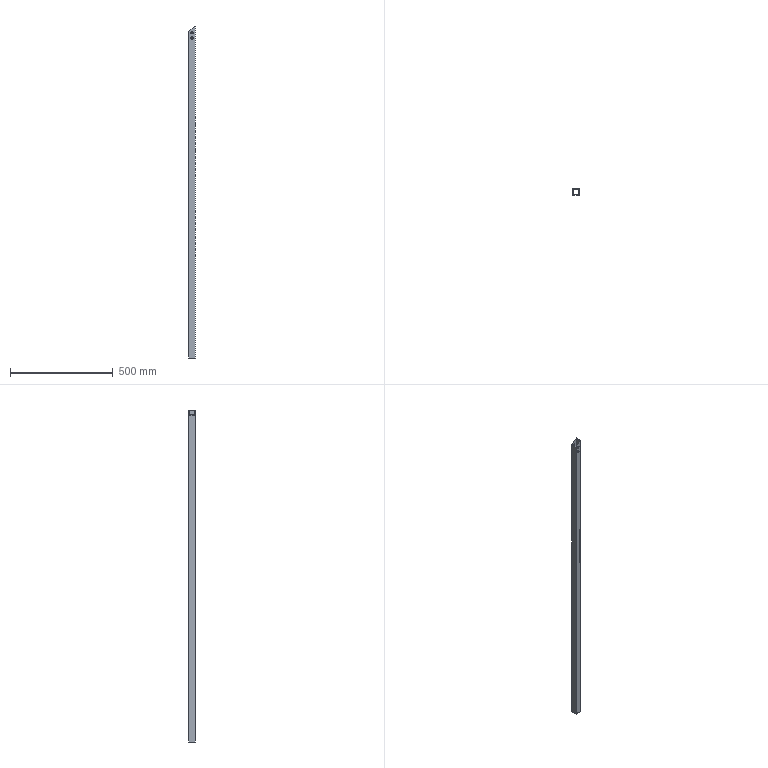Part | SolidWorks | features Cut 1, Extrusion 1, ICE 1 | 1 solid | 18 faces | box 30 x 30 x 1612 mm | volume 357438 mm3 | plane 10 | cylinder 8 | commonest cylinder face diameters 11.5 x8
STEP:
#1=CARTESIAN_POINT('',(-5.75,15.,745.414));
#2=VERTEX_POINT('',#1);
#3=CARTESIAN_POINT('',(5.75,15.,745.414));
#4=VERTEX_POINT('',#3);
#5=CARTESIAN_POINT('',(0.,15.,745.414));
#6=DIRECTION('',(0.,-1.,0.));
#7=DIRECTION('',(0.,0.,-1.));
#8=AXIS2_PLACEMENT_3D('',#5,#6,#7);
#9=CIRCLE('',#8,5.75);
#10=EDGE_CURVE('',#2,#4,#9,.T.);
#11=ORIENTED_EDGE('',*,*,#10,.F.);
#12=CARTESIAN_POINT('',(-5.75,13.,745.414));
#13=VERTEX_POINT('',#12);
#14=CARTESIAN_POINT('',(-5.75,148.,745.414));
#15=DIRECTION('',(0.,-1.,0.));
#16=VECTOR('',#15,1000.);
#17=LINE('',#14,#16);
#18=EDGE_CURVE('',#2,#13,#17,.T.);
#19=ORIENTED_EDGE('',*,*,#18,.T.);
#20=CARTESIAN_POINT('',(5.75,13.,745.414));
#21=VERTEX_POINT('',#20);
#22=CARTESIAN_POINT('',(0.,13.,745.414));
#23=DIRECTION('',(0.,-1.,0.));
#24=DIRECTION('',(0.,0.,-1.));
#25=AXIS2_PLACEMENT_3D('',#22,#23,#24);
#26=CIRCLE('',#25,5.75);
#27=EDGE_CURVE('',#13,#21,#26,.T.);
#28=ORIENTED_EDGE('',*,*,#27,.T.);
#29=CARTESIAN_POINT('',(5.75,148.,745.414));
#30=DIRECTION('',(0.,-1.,0.));
#31=VECTOR('',#30,1000.);
#32=LINE('',#29,#31);
#33=EDGE_CURVE('',#4,#21,#32,.T.);
#34=ORIENTED_EDGE('',*,*,#33,.F.);
#35=EDGE_LOOP('',(#11,#19,#28,#34));
#36=FACE_OUTER_BOUND('',#35,.T.);
#37=CARTESIAN_POINT('',(0.,148.,745.414));
#38=DIRECTION('',(0.,-1.,0.));
#39=DIRECTION('',(1.,0.,0.));
#40=AXIS2_PLACEMENT_3D('',#37,#38,#39);
#41=CYLINDRICAL_SURFACE('',#40,5.75);
#42=ADVANCED_FACE('',(#36),#41,.F.);
#43=CARTESIAN_POINT('',(-5.75,15.,720.414));
#44=VERTEX_POINT('',#43);
#45=CARTESIAN_POINT('',(5.75,15.,720.414));
#46=VERTEX_POINT('',#45);
#47=CARTESIAN_POINT('',(0.,15.,720.414));
#48=DIRECTION('',(0.,-1.,0.));
#49=DIRECTION('',(0.,0.,-1.));
#50=AXIS2_PLACEMENT_3D('',#47,#48,#49);
#51=CIRCLE('',#50,5.75);
#52=EDGE_CURVE('',#44,#46,#51,.T.);
#53=ORIENTED_EDGE('',*,*,#52,.F.);
#54=CARTESIAN_POINT('',(-5.75,13.,720.414));
#55=VERTEX_POINT('',#54);
#56=CARTESIAN_POINT('',(-5.75,148.,720.414));
#57=DIRECTION('',(0.,-1.,0.));
#58=VECTOR('',#57,1000.);
#59=LINE('',#56,#58);
#60=EDGE_CURVE('',#44,#55,#59,.T.);
#61=ORIENTED_EDGE('',*,*,#60,.T.);
#62=CARTESIAN_POINT('',(5.75,13.,720.414));
#63=VERTEX_POINT('',#62);
#64=CARTESIAN_POINT('',(0.,13.,720.414));
#65=DIRECTION('',(0.,-1.,0.));
#66=DIRECTION('',(0.,0.,-1.));
#67=AXIS2_PLACEMENT_3D('',#64,#65,#66);
#68=CIRCLE('',#67,5.75);
#69=EDGE_CURVE('',#55,#63,#68,.T.);
#70=ORIENTED_EDGE('',*,*,#69,.T.);
#71=CARTESIAN_POINT('',(5.75,148.,720.414));
#72=DIRECTION('',(0.,-1.,0.));
#73=VECTOR('',#72,1000.);
#74=LINE('',#71,#73);
#75=EDGE_CURVE('',#46,#63,#74,.T.);
#76=ORIENTED_EDGE('',*,*,#75,.F.);
#77=EDGE_LOOP('',(#53,#61,#70,#76));
#78=FACE_OUTER_BOUND('',#77,.T.);
#79=CARTESIAN_POINT('',(0.,148.,720.414));
#80=DIRECTION('',(0.,-1.,0.));
#81=DIRECTION('',(1.,0.,0.));
#82=AXIS2_PLACEMENT_3D('',#79,#80,#81);
#83=CYLINDRICAL_SURFACE('',#82,5.75);
#84=ADVANCED_FACE('',(#78),#83,.F.);
#85=CARTESIAN_POINT('',(5.75,-13.,745.414));
#86=VERTEX_POINT('',#85);
#87=CARTESIAN_POINT('',(-5.75,-13.,745.414));
#88=VERTEX_POINT('',#87);
#89=CARTESIAN_POINT('',(0.,-13.,745.414));
#90=DIRECTION('',(0.,1.,0.));
#91=DIRECTION('',(0.,0.,1.));
#92=AXIS2_PLACEMENT_3D('',#89,#90,#91);
#93=CIRCLE('',#92,5.75);
#94=EDGE_CURVE('',#86,#88,#93,.T.);
#95=ORIENTED_EDGE('',*,*,#94,.T.);
#96=CARTESIAN_POINT('',(-5.75,-15.,745.414));
#97=VERTEX_POINT('',#96);
#98=CARTESIAN_POINT('',(-5.75,148.,745.414));
#99=DIRECTION('',(0.,-1.,0.));
#100=VECTOR('',#99,1000.);
#101=LINE('',#98,#100);
#102=EDGE_CURVE('',#88,#97,#101,.T.);
#103=ORIENTED_EDGE('',*,*,#102,.T.);
#104=CARTESIAN_POINT('',(5.75,-15.,745.414));
#105=VERTEX_POINT('',#104);
#106=CARTESIAN_POINT('',(0.,-15.,745.414));
#107=DIRECTION('',(0.,-1.,0.));
#108=DIRECTION('',(1.,0.,0.));
#109=AXIS2_PLACEMENT_3D('',#106,#107,#108);
#110=CIRCLE('',#109,5.75);
#111=EDGE_CURVE('',#97,#105,#110,.T.);
#112=ORIENTED_EDGE('',*,*,#111,.T.);
#113=CARTESIAN_POINT('',(5.75,148.,745.414));
#114=DIRECTION('',(0.,-1.,0.));
#115=VECTOR('',#114,1000.);
#116=LINE('',#113,#115);
#117=EDGE_CURVE('',#86,#105,#116,.T.);
#118=ORIENTED_EDGE('',*,*,#117,.F.);
#119=EDGE_LOOP('',(#95,#103,#112,#118));
#120=FACE_OUTER_BOUND('',#119,.T.);
#121=CARTESIAN_POINT('',(0.,148.,745.414));
#122=DIRECTION('',(0.,-1.,0.));
#123=DIRECTION('',(1.,0.,0.));
#124=AXIS2_PLACEMENT_3D('',#121,#122,#123);
#125=CYLINDRICAL_SURFACE('',#124,5.75);
#126=ADVANCED_FACE('',(#120),#125,.F.);
#127=CARTESIAN_POINT('',(5.75,-13.,720.414));
#128=VERTEX_POINT('',#127);
#129=CARTESIAN_POINT('',(-5.75,-13.,720.414));
#130=VERTEX_POINT('',#129);
#131=CARTESIAN_POINT('',(0.,-13.,720.414));
#132=DIRECTION('',(0.,1.,0.));
#133=DIRECTION('',(0.,0.,1.));
#134=AXIS2_PLACEMENT_3D('',#131,#132,#133);
#135=CIRCLE('',#134,5.75);
#136=EDGE_CURVE('',#128,#130,#135,.T.);
#137=ORIENTED_EDGE('',*,*,#136,.T.);
#138=CARTESIAN_POINT('',(-5.75,-15.,720.414));
#139=VERTEX_POINT('',#138);
#140=CARTESIAN_POINT('',(-5.75,148.,720.414));
#141=DIRECTION('',(0.,-1.,0.));
#142=VECTOR('',#141,1000.);
#143=LINE('',#140,#142);
#144=EDGE_CURVE('',#130,#139,#143,.T.);
#145=ORIENTED_EDGE('',*,*,#144,.T.);
#146=CARTESIAN_POINT('',(5.75,-15.,720.414));
#147=VERTEX_POINT('',#146);
#148=CARTESIAN_POINT('',(0.,-15.,720.414));
#149=DIRECTION('',(0.,-1.,0.));
#150=DIRECTION('',(1.,0.,0.));
#151=AXIS2_PLACEMENT_3D('',#148,#149,#150);
#152=CIRCLE('',#151,5.75);
#153=EDGE_CURVE('',#139,#147,#152,.T.);
#154=ORIENTED_EDGE('',*,*,#153,.T.);
#155=CARTESIAN_POINT('',(5.75,148.,720.414));
#156=DIRECTION('',(0.,-1.,0.));
#157=VECTOR('',#156,1000.);
#158=LINE('',#155,#157);
#159=EDGE_CURVE('',#128,#147,#158,.T.);
#160=ORIENTED_EDGE('',*,*,#159,.F.);
#161=EDGE_LOOP('',(#137,#145,#154,#160));
#162=FACE_OUTER_BOUND('',#161,.T.);
#163=CARTESIAN_POINT('',(0.,148.,720.414));
#164=DIRECTION('',(0.,-1.,0.));
#165=DIRECTION('',(1.,0.,0.));
#166=AXIS2_PLACEMENT_3D('',#163,#164,#165);
#167=CYLINDRICAL_SURFACE('',#166,5.75);
#168=ADVANCED_FACE('',(#162),#167,.F.);
#169=CARTESIAN_POINT('',(-15.,15.,-833.5));
#170=VERTEX_POINT('',#169);
#171=CARTESIAN_POINT('',(-15.,-15.,-833.5));
#172=VERTEX_POINT('',#171);
#173=CARTESIAN_POINT('',(-15.,-15.,-833.5));
#174=DIRECTION('',(0.,-1.,0.));
#175=VECTOR('',#174,1000.);
#176=LINE('',#173,#175);
#177=EDGE_CURVE('',#170,#172,#176,.T.);
#178=ORIENTED_EDGE('',*,*,#177,.F.);
#179=CARTESIAN_POINT('',(15.,15.,-833.5));
#180=VERTEX_POINT('',#179);
#181=CARTESIAN_POINT('',(15.,15.,-833.5));
#182=DIRECTION('',(-1.,0.,0.));
#183=VECTOR('',#182,1000.);
#184=LINE('',#181,#183);
#185=EDGE_CURVE('',#180,#170,#184,.T.);
#186=ORIENTED_EDGE('',*,*,#185,.F.);
#187=CARTESIAN_POINT('',(15.,-15.,-833.5));
#188=VERTEX_POINT('',#187);
#189=CARTESIAN_POINT('',(15.,-15.,-833.5));
#190=DIRECTION('',(0.,1.,0.));
#191=VECTOR('',#190,1000.);
#192=LINE('',#189,#191);
#193=EDGE_CURVE('',#188,#180,#192,.T.);
#194=ORIENTED_EDGE('',*,*,#193,.F.);
#195=CARTESIAN_POINT('',(15.,-15.,-833.5));
#196=DIRECTION('',(1.,0.,0.));
#197=VECTOR('',#196,1000.);
#198=LINE('',#195,#197);
#199=EDGE_CURVE('',#172,#188,#198,.T.);
#200=ORIENTED_EDGE('',*,*,#199,.F.);
#201=EDGE_LOOP('',(#178,#186,#194,#200));
#202=FACE_OUTER_BOUND('',#201,.T.);
#203=CARTESIAN_POINT('',(13.,-13.,-833.5));
#204=VERTEX_POINT('',#203);
#205=CARTESIAN_POINT('',(13.,13.,-833.5));
#206=VERTEX_POINT('',#205);
#207=CARTESIAN_POINT('',(13.,-13.,-833.5));
#208=DIRECTION('',(0.,1.,0.));
#209=VECTOR('',#208,1000.);
#210=LINE('',#207,#209);
#211=EDGE_CURVE('',#204,#206,#210,.T.);
#212=ORIENTED_EDGE('',*,*,#211,.T.);
#213=CARTESIAN_POINT('',(-13.,13.,-833.5));
#214=VERTEX_POINT('',#213);
#215=CARTESIAN_POINT('',(13.,13.,-833.5));
#216=DIRECTION('',(-1.,0.,0.));
#217=VECTOR('',#216,1000.);
#218=LINE('',#215,#217);
#219=EDGE_CURVE('',#206,#214,#218,.T.);
#220=ORIENTED_EDGE('',*,*,#219,.T.);
#221=CARTESIAN_POINT('',(-13.,-13.,-833.5));
#222=VERTEX_POINT('',#221);
#223=CARTESIAN_POINT('',(-13.,-13.,-833.5));
#224=DIRECTION('',(0.,-1.,0.));
#225=VECTOR('',#224,1000.);
#226=LINE('',#223,#225);
#227=EDGE_CURVE('',#214,#222,#226,.T.);
#228=ORIENTED_EDGE('',*,*,#227,.T.);
#229=CARTESIAN_POINT('',(13.,-13.,-833.5));
#230=DIRECTION('',(1.,0.,0.));
#231=VECTOR('',#230,1000.);
#232=LINE('',#229,#231);
#233=EDGE_CURVE('',#222,#204,#232,.T.);
#234=ORIENTED_EDGE('',*,*,#233,.T.);
#235=EDGE_LOOP('',(#212,#220,#228,#234));
#236=FACE_BOUND('',#235,.T.);
#237=CARTESIAN_POINT('',(0.,0.,-833.5));
#238=DIRECTION('',(0.,0.,1.));
#239=DIRECTION('',(1.,0.,0.));
#240=AXIS2_PLACEMENT_3D('',#237,#238,#239);
#241=PLANE('',#240);
#242=ADVANCED_FACE('',(#202,#236),#241,.F.);
#243=CARTESIAN_POINT('',(-15.,-15.,753.327));
#244=VERTEX_POINT('',#243);
#245=CARTESIAN_POINT('',(-15.,-15.,833.5));
#246=DIRECTION('',(0.,0.,-1.));
#247=VECTOR('',#246,1000.);
#248=LINE('',#245,#247);
#249=EDGE_CURVE('',#244,#172,#248,.T.);
#250=ORIENTED_EDGE('',*,*,#249,.F.);
#251=CARTESIAN_POINT('',(-15.,15.,753.327));
#252=VERTEX_POINT('',#251);
#253=CARTESIAN_POINT('',(-15.,-20.,753.327));
#254=DIRECTION('',(0.,1.,0.));
#255=VECTOR('',#254,1000.);
#256=LINE('',#253,#255);
#257=EDGE_CURVE('',#244,#252,#256,.T.);
#258=ORIENTED_EDGE('',*,*,#257,.T.);
#259=CARTESIAN_POINT('',(-15.,15.,833.5));
#260=DIRECTION('',(0.,0.,-1.));
#261=VECTOR('',#260,1000.);
#262=LINE('',#259,#261);
#263=EDGE_CURVE('',#252,#170,#262,.T.);
#264=ORIENTED_EDGE('',*,*,#263,.T.);
#265=ORIENTED_EDGE('',*,*,#177,.T.);
#266=EDGE_LOOP('',(#250,#258,#264,#265));
#267=FACE_OUTER_BOUND('',#266,.T.);
#268=CARTESIAN_POINT('',(-15.,-15.,833.5));
#269=DIRECTION('',(1.,0.,0.));
#270=DIRECTION('',(0.,1.,0.));
#271=AXIS2_PLACEMENT_3D('',#268,#269,#270);
#272=PLANE('',#271);
#273=ADVANCED_FACE('',(#267),#272,.F.);
#274=CARTESIAN_POINT('',(0.,-15.,745.414));
#275=DIRECTION('',(0.,-1.,0.));
#276=DIRECTION('',(1.,0.,0.));
#277=AXIS2_PLACEMENT_3D('',#274,#275,#276);
#278=CIRCLE('',#277,5.75);
#279=EDGE_CURVE('',#105,#97,#278,.T.);
#280=ORIENTED_EDGE('',*,*,#279,.F.);
#281=ORIENTED_EDGE('',*,*,#111,.F.);
#282=EDGE_LOOP('',(#280,#281));
#283=FACE_BOUND('',#282,.T.);
#284=CARTESIAN_POINT('',(0.,-15.,720.414));
#285=DIRECTION('',(0.,-1.,0.));
#286=DIRECTION('',(1.,0.,0.));
#287=AXIS2_PLACEMENT_3D('',#284,#285,#286);
#288=CIRCLE('',#287,5.75);
#289=EDGE_CURVE('',#147,#139,#288,.T.);
#290=ORIENTED_EDGE('',*,*,#289,.F.);
#291=ORIENTED_EDGE('',*,*,#153,.F.);
#292=EDGE_LOOP('',(#290,#291));
#293=FACE_BOUND('',#292,.T.);
#294=CARTESIAN_POINT('',(15.,-15.,778.5));
#295=VERTEX_POINT('',#294);
#296=CARTESIAN_POINT('',(15.,-15.,833.5));
#297=DIRECTION('',(0.,0.,-1.));
#298=VECTOR('',#297,1000.);
#299=LINE('',#296,#298);
#300=EDGE_CURVE('',#295,#188,#299,.T.);
#301=ORIENTED_EDGE('',*,*,#300,.F.);
#302=CARTESIAN_POINT('',(42.082,-15.,801.225));
#303=DIRECTION('',(-0.766,0.,-0.6428));
#304=VECTOR('',#303,1000.);
#305=LINE('',#302,#304);
#306=EDGE_CURVE('',#295,#244,#305,.T.);
#307=ORIENTED_EDGE('',*,*,#306,.T.);
#308=ORIENTED_EDGE('',*,*,#249,.T.);
#309=ORIENTED_EDGE('',*,*,#199,.T.);
#310=EDGE_LOOP('',(#301,#307,#308,#309));
#311=FACE_OUTER_BOUND('',#310,.T.);
#312=CARTESIAN_POINT('',(15.,-15.,833.5));
#313=DIRECTION('',(0.,1.,0.));
#314=DIRECTION('',(-1.,0.,0.));
#315=AXIS2_PLACEMENT_3D('',#312,#313,#314);
#316=PLANE('',#315);
#317=ADVANCED_FACE('',(#283,#293,#311),#316,.F.);
#318=CARTESIAN_POINT('',(15.,15.,778.5));
#319=VERTEX_POINT('',#318);
#320=CARTESIAN_POINT('',(15.,15.,833.5));
#321=DIRECTION('',(0.,0.,-1.));
#322=VECTOR('',#321,1000.);
#323=LINE('',#320,#322);
#324=EDGE_CURVE('',#319,#180,#323,.T.);
#325=ORIENTED_EDGE('',*,*,#324,.F.);
#326=CARTESIAN_POINT('',(15.,-20.,778.5));
#327=DIRECTION('',(0.,1.,0.));
#328=VECTOR('',#327,1000.);
#329=LINE('',#326,#328);
#330=EDGE_CURVE('',#295,#319,#329,.T.);
#331=ORIENTED_EDGE('',*,*,#330,.F.);
#332=ORIENTED_EDGE('',*,*,#300,.T.);
#333=ORIENTED_EDGE('',*,*,#193,.T.);
#334=EDGE_LOOP('',(#325,#331,#332,#333));
#335=FACE_OUTER_BOUND('',#334,.T.);
#336=CARTESIAN_POINT('',(15.,-15.,833.5));
#337=DIRECTION('',(-1.,0.,0.));
#338=DIRECTION('',(0.,0.,1.));
#339=AXIS2_PLACEMENT_3D('',#336,#337,#338);
#340=PLANE('',#339);
#341=ADVANCED_FACE('',(#335),#340,.F.);
#342=CARTESIAN_POINT('',(0.,15.,745.414));
#343=DIRECTION('',(0.,-1.,0.));
#344=DIRECTION('',(0.,0.,-1.));
#345=AXIS2_PLACEMENT_3D('',#342,#343,#344);
#346=CIRCLE('',#345,5.75);
#347=EDGE_CURVE('',#4,#2,#346,.T.);
#348=ORIENTED_EDGE('',*,*,#347,.T.);
#349=ORIENTED_EDGE('',*,*,#10,.T.);
#350=EDGE_LOOP('',(#348,#349));
#351=FACE_BOUND('',#350,.T.);
#352=CARTESIAN_POINT('',(0.,15.,720.414));
#353=DIRECTION('',(0.,-1.,0.));
#354=DIRECTION('',(0.,0.,-1.));
#355=AXIS2_PLACEMENT_3D('',#352,#353,#354);
#356=CIRCLE('',#355,5.75);
#357=EDGE_CURVE('',#46,#44,#356,.T.);
#358=ORIENTED_EDGE('',*,*,#357,.T.);
#359=ORIENTED_EDGE('',*,*,#52,.T.);
#360=EDGE_LOOP('',(#358,#359));
#361=FACE_BOUND('',#360,.T.);
#362=ORIENTED_EDGE('',*,*,#263,.F.);
#363=CARTESIAN_POINT('',(42.082,15.,801.225));
#364=DIRECTION('',(0.766,0.,0.6428));
#365=VECTOR('',#364,1000.);
#366=LINE('',#363,#365);
#367=EDGE_CURVE('',#252,#319,#366,.T.);
#368=ORIENTED_EDGE('',*,*,#367,.T.);
#369=ORIENTED_EDGE('',*,*,#324,.T.);
#370=ORIENTED_EDGE('',*,*,#185,.T.);
#371=EDGE_LOOP('',(#362,#368,#369,#370));
#372=FACE_OUTER_BOUND('',#371,.T.);
#373=CARTESIAN_POINT('',(15.,15.,833.5));
#374=DIRECTION('',(0.,-1.,0.));
#375=DIRECTION('',(0.,0.,-1.));
#376=AXIS2_PLACEMENT_3D('',#373,#374,#375);
#377=PLANE('',#376);
#378=ADVANCED_FACE('',(#351,#361,#372),#377,.F.);
#379=CARTESIAN_POINT('',(13.,13.,776.822));
#380=VERTEX_POINT('',#379);
#381=CARTESIAN_POINT('',(13.,-13.,776.822));
#382=VERTEX_POINT('',#381);
#383=CARTESIAN_POINT('',(13.,-13.,776.822));
#384=DIRECTION('',(0.,-1.,0.));
#385=VECTOR('',#384,1000.);
#386=LINE('',#383,#385);
#387=EDGE_CURVE('',#380,#382,#386,.T.);
#388=ORIENTED_EDGE('',*,*,#387,.F.);
#389=CARTESIAN_POINT('',(13.,13.,833.5));
#390=DIRECTION('',(0.,0.,-1.));
#391=VECTOR('',#390,1000.);
#392=LINE('',#389,#391);
#393=EDGE_CURVE('',#380,#206,#392,.T.);
#394=ORIENTED_EDGE('',*,*,#393,.T.);
#395=ORIENTED_EDGE('',*,*,#211,.F.);
#396=CARTESIAN_POINT('',(13.,-13.,833.5));
#397=DIRECTION('',(0.,0.,-1.));
#398=VECTOR('',#397,1000.);
#399=LINE('',#396,#398);
#400=EDGE_CURVE('',#382,#204,#399,.T.);
#401=ORIENTED_EDGE('',*,*,#400,.F.);
#402=EDGE_LOOP('',(#388,#394,#395,#401));
#403=FACE_OUTER_BOUND('',#402,.T.);
#404=CARTESIAN_POINT('',(13.,-13.,833.5));
#405=DIRECTION('',(-1.,0.,0.));
#406=DIRECTION('',(0.,0.,1.));
#407=AXIS2_PLACEMENT_3D('',#404,#405,#406);
#408=PLANE('',#407);
#409=ADVANCED_FACE('',(#403),#408,.T.);
#410=CARTESIAN_POINT('',(0.,13.,745.414));
#411=DIRECTION('',(0.,-1.,0.));
#412=DIRECTION('',(0.,0.,-1.));
#413=AXIS2_PLACEMENT_3D('',#410,#411,#412);
#414=CIRCLE('',#413,5.75);
#415=EDGE_CURVE('',#21,#13,#414,.T.);
#416=ORIENTED_EDGE('',*,*,#415,.F.);
#417=ORIENTED_EDGE('',*,*,#27,.F.);
#418=EDGE_LOOP('',(#416,#417));
#419=FACE_BOUND('',#418,.T.);
#420=CARTESIAN_POINT('',(0.,13.,720.414));
#421=DIRECTION('',(0.,-1.,0.));
#422=DIRECTION('',(0.,0.,-1.));
#423=AXIS2_PLACEMENT_3D('',#420,#421,#422);
#424=CIRCLE('',#423,5.75);
#425=EDGE_CURVE('',#63,#55,#424,.T.);
#426=ORIENTED_EDGE('',*,*,#425,.F.);
#427=ORIENTED_EDGE('',*,*,#69,.F.);
#428=EDGE_LOOP('',(#426,#427));
#429=FACE_BOUND('',#428,.T.);
#430=CARTESIAN_POINT('',(-13.,13.,755.005));
#431=VERTEX_POINT('',#430);
#432=CARTESIAN_POINT('',(40.909,13.,800.24));
#433=DIRECTION('',(0.766,0.,0.6428));
#434=VECTOR('',#433,1000.);
#435=LINE('',#432,#434);
#436=EDGE_CURVE('',#431,#380,#435,.T.);
#437=ORIENTED_EDGE('',*,*,#436,.F.);
#438=CARTESIAN_POINT('',(-13.,13.,833.5));
#439=DIRECTION('',(0.,0.,-1.));
#440=VECTOR('',#439,1000.);
#441=LINE('',#438,#440);
#442=EDGE_CURVE('',#431,#214,#441,.T.);
#443=ORIENTED_EDGE('',*,*,#442,.T.);
#444=ORIENTED_EDGE('',*,*,#219,.F.);
#445=ORIENTED_EDGE('',*,*,#393,.F.);
#446=EDGE_LOOP('',(#437,#443,#444,#445));
#447=FACE_OUTER_BOUND('',#446,.T.);
#448=CARTESIAN_POINT('',(13.,13.,833.5));
#449=DIRECTION('',(0.,-1.,0.));
#450=DIRECTION('',(0.,0.,-1.));
#451=AXIS2_PLACEMENT_3D('',#448,#449,#450);
#452=PLANE('',#451);
#453=ADVANCED_FACE('',(#419,#429,#447),#452,.T.);
#454=CARTESIAN_POINT('',(-13.,-13.,755.005));
#455=VERTEX_POINT('',#454);
#456=CARTESIAN_POINT('',(-13.,-13.,755.005));
#457=DIRECTION('',(0.,1.,0.));
#458=VECTOR('',#457,1000.);
#459=LINE('',#456,#458);
#460=EDGE_CURVE('',#455,#431,#459,.T.);
#461=ORIENTED_EDGE('',*,*,#460,.F.);
#462=CARTESIAN_POINT('',(-13.,-13.,833.5));
#463=DIRECTION('',(0.,0.,-1.));
#464=VECTOR('',#463,1000.);
#465=LINE('',#462,#464);
#466=EDGE_CURVE('',#455,#222,#465,.T.);
#467=ORIENTED_EDGE('',*,*,#466,.T.);
#468=ORIENTED_EDGE('',*,*,#227,.F.);
#469=ORIENTED_EDGE('',*,*,#442,.F.);
#470=EDGE_LOOP('',(#461,#467,#468,#469));
#471=FACE_OUTER_BOUND('',#470,.T.);
#472=CARTESIAN_POINT('',(-13.,-13.,833.5));
#473=DIRECTION('',(1.,0.,0.));
#474=DIRECTION('',(0.,0.,-1.));
#475=AXIS2_PLACEMENT_3D('',#472,#473,#474);
#476=PLANE('',#475);
#477=ADVANCED_FACE('',(#471),#476,.T.);
#478=ORIENTED_EDGE('',*,*,#94,.F.);
#479=CARTESIAN_POINT('',(0.,-13.,745.414));
#480=DIRECTION('',(0.,1.,0.));
#481=DIRECTION('',(0.,0.,1.));
#482=AXIS2_PLACEMENT_3D('',#479,#480,#481);
#483=CIRCLE('',#482,5.75);
#484=EDGE_CURVE('',#88,#86,#483,.T.);
#485=ORIENTED_EDGE('',*,*,#484,.F.);
#486=EDGE_LOOP('',(#478,#485));
#487=FACE_BOUND('',#486,.T.);
#488=ORIENTED_EDGE('',*,*,#136,.F.);
#489=CARTESIAN_POINT('',(0.,-13.,720.414));
#490=DIRECTION('',(0.,1.,0.));
#491=DIRECTION('',(0.,0.,1.));
#492=AXIS2_PLACEMENT_3D('',#489,#490,#491);
#493=CIRCLE('',#492,5.75);
#494=EDGE_CURVE('',#130,#128,#493,.T.);
#495=ORIENTED_EDGE('',*,*,#494,.F.);
#496=EDGE_LOOP('',(#488,#495));
#497=FACE_BOUND('',#496,.T.);
#498=CARTESIAN_POINT('',(40.909,-13.,800.24));
#499=DIRECTION('',(-0.766,0.,-0.6428));
#500=VECTOR('',#499,1000.);
#501=LINE('',#498,#500);
#502=EDGE_CURVE('',#382,#455,#501,.T.);
#503=ORIENTED_EDGE('',*,*,#502,.F.);
#504=ORIENTED_EDGE('',*,*,#400,.T.);
#505=ORIENTED_EDGE('',*,*,#233,.F.);
#506=ORIENTED_EDGE('',*,*,#466,.F.);
#507=EDGE_LOOP('',(#503,#504,#505,#506));
#508=FACE_OUTER_BOUND('',#507,.T.);
#509=CARTESIAN_POINT('',(13.,-13.,833.5));
#510=DIRECTION('',(0.,1.,0.));
#511=DIRECTION('',(0.,0.,1.));
#512=AXIS2_PLACEMENT_3D('',#509,#510,#511);
#513=PLANE('',#512);
#514=ADVANCED_FACE('',(#487,#497,#508),#513,.T.);
#515=ORIENTED_EDGE('',*,*,#387,.T.);
#516=ORIENTED_EDGE('',*,*,#502,.T.);
#517=ORIENTED_EDGE('',*,*,#460,.T.);
#518=ORIENTED_EDGE('',*,*,#436,.T.);
#519=EDGE_LOOP('',(#515,#516,#517,#518));
#520=FACE_BOUND('',#519,.T.);
#521=ORIENTED_EDGE('',*,*,#330,.T.);
#522=ORIENTED_EDGE('',*,*,#367,.F.);
#523=ORIENTED_EDGE('',*,*,#257,.F.);
#524=ORIENTED_EDGE('',*,*,#306,.F.);
#525=EDGE_LOOP('',(#521,#522,#523,#524));
#526=FACE_OUTER_BOUND('',#525,.T.);
#527=CARTESIAN_POINT('',(-377.139,-20.,449.456));
#528=DIRECTION('',(0.6428,0.,-0.766));
#529=DIRECTION('',(-0.766,0.,-0.6428));
#530=AXIS2_PLACEMENT_3D('',#527,#528,#529);
#531=PLANE('',#530);
#532=ADVANCED_FACE('',(#520,#526),#531,.F.);
#533=ORIENTED_EDGE('',*,*,#144,.F.);
#534=ORIENTED_EDGE('',*,*,#494,.T.);
#535=ORIENTED_EDGE('',*,*,#159,.T.);
#536=ORIENTED_EDGE('',*,*,#289,.T.);
#537=EDGE_LOOP('',(#533,#534,#535,#536));
#538=FACE_OUTER_BOUND('',#537,.T.);
#539=CARTESIAN_POINT('',(0.,148.,720.414));
#540=DIRECTION('',(0.,-1.,0.));
#541=DIRECTION('',(1.,0.,0.));
#542=AXIS2_PLACEMENT_3D('',#539,#540,#541);
#543=CYLINDRICAL_SURFACE('',#542,5.75);
#544=ADVANCED_FACE('',(#538),#543,.F.);
#545=ORIENTED_EDGE('',*,*,#102,.F.);
#546=ORIENTED_EDGE('',*,*,#484,.T.);
#547=ORIENTED_EDGE('',*,*,#117,.T.);
#548=ORIENTED_EDGE('',*,*,#279,.T.);
#549=EDGE_LOOP('',(#545,#546,#547,#548));
#550=FACE_OUTER_BOUND('',#549,.T.);
#551=CARTESIAN_POINT('',(0.,148.,745.414));
#552=DIRECTION('',(0.,-1.,0.));
#553=DIRECTION('',(1.,0.,0.));
#554=AXIS2_PLACEMENT_3D('',#551,#552,#553);
#555=CYLINDRICAL_SURFACE('',#554,5.75);
#556=ADVANCED_FACE('',(#550),#555,.F.);
#557=ORIENTED_EDGE('',*,*,#60,.F.);
#558=ORIENTED_EDGE('',*,*,#357,.F.);
#559=ORIENTED_EDGE('',*,*,#75,.T.);
#560=ORIENTED_EDGE('',*,*,#425,.T.);
#561=EDGE_LOOP('',(#557,#558,#559,#560));
#562=FACE_OUTER_BOUND('',#561,.T.);
#563=CARTESIAN_POINT('',(0.,148.,720.414));
#564=DIRECTION('',(0.,-1.,0.));
#565=DIRECTION('',(1.,0.,0.));
#566=AXIS2_PLACEMENT_3D('',#563,#564,#565);
#567=CYLINDRICAL_SURFACE('',#566,5.75);
#568=ADVANCED_FACE('',(#562),#567,.F.);
#569=ORIENTED_EDGE('',*,*,#18,.F.);
#570=ORIENTED_EDGE('',*,*,#347,.F.);
#571=ORIENTED_EDGE('',*,*,#33,.T.);
#572=ORIENTED_EDGE('',*,*,#415,.T.);
#573=EDGE_LOOP('',(#569,#570,#571,#572));
#574=FACE_OUTER_BOUND('',#573,.T.);
#575=CARTESIAN_POINT('',(0.,148.,745.414));
#576=DIRECTION('',(0.,-1.,0.));
#577=DIRECTION('',(1.,0.,0.));
#578=AXIS2_PLACEMENT_3D('',#575,#576,#577);
#579=CYLINDRICAL_SURFACE('',#578,5.75);
#580=ADVANCED_FACE('',(#574),#579,.F.);
#581=CLOSED_SHELL('',(#42,#84,#126,#168,#242,#273,#317,#341,#378,#409,#453,#477,#514,#532,#544,#556,#568,#580));
#582=MANIFOLD_SOLID_BREP('',#581);
#583=CARTESIAN_POINT('',(0.,0.,0.));
#584=DIRECTION('',(0.,0.,1.));
#585=DIRECTION('',(1.,0.,0.));
#586=AXIS2_PLACEMENT_3D('',#583,#584,#585);
#587=(LENGTH_UNIT()NAMED_UNIT(*)SI_UNIT(.MILLI.,.METRE.));
#588=UNCERTAINTY_MEASURE_WITH_UNIT(LENGTH_MEASURE(0.00001),#587,'','');
#589=(NAMED_UNIT(*)PLANE_ANGLE_UNIT()SI_UNIT($,.RADIAN.));
#590=(NAMED_UNIT(*)SI_UNIT($,.STERADIAN.)SOLID_ANGLE_UNIT());
#591=(GEOMETRIC_REPRESENTATION_CONTEXT(3)GLOBAL_UNCERTAINTY_ASSIGNED_CONTEXT((#588))GLOBAL_UNIT_ASSIGNED_CONTEXT((#587,#589,#590))REPRESENTATION_CONTEXT('',''));
#592=ADVANCED_BREP_SHAPE_REPRESENTATION('',(#582,#586),#591);